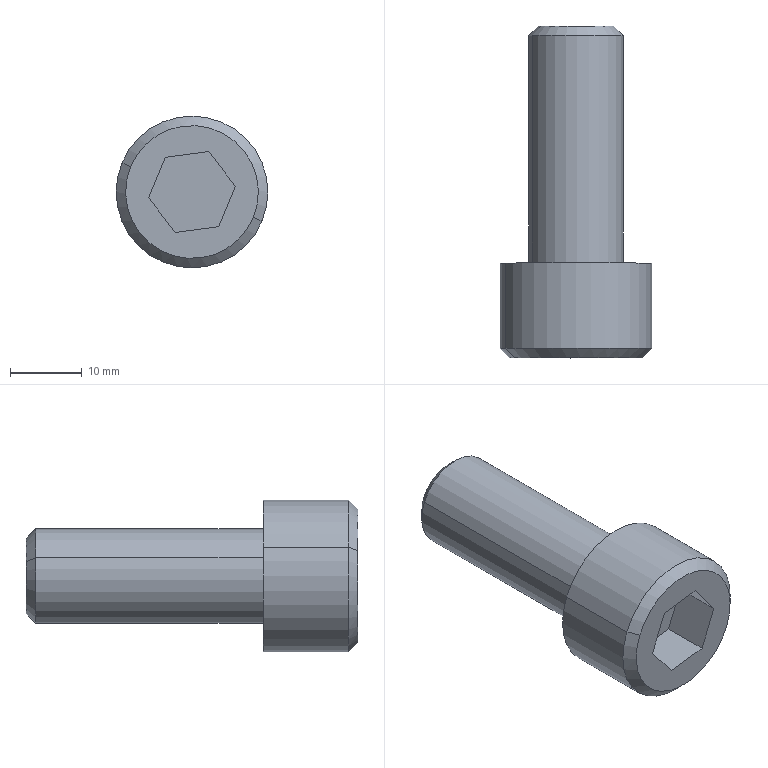Part | SolidWorks | features BaseBody 1 | 1 solid | 18 faces | box 21.12 x 46.2 x 21.12 mm | volume 8414 mm3 | plane 10 | cone 4 | cylinder 4 | commonest cylinder face diameters 13.2 x2 21.12 x2
STEP:
#1=CARTESIAN_POINT('',(-2171.446,543.257,-1544.855));
#2=VERTEX_POINT('',#1);
#3=CARTESIAN_POINT('',(-2170.226,541.937,-1545.359));
#4=VERTEX_POINT('',#3);
#5=CARTESIAN_POINT('',(-2171.446,543.257,-1544.855));
#6=DIRECTION('',(0.6535,-0.7071,-0.27));
#7=VECTOR('',#6,1000.);
#8=LINE('',#5,#7);
#9=EDGE_CURVE('',#2,#4,#8,.T.);
#10=ORIENTED_EDGE('',*,*,#9,.T.);
#11=CARTESIAN_POINT('',(-2153.147,541.937,-1552.416));
#12=VERTEX_POINT('',#11);
#13=CARTESIAN_POINT('',(-2161.687,541.937,-1548.888));
#14=DIRECTION('',(0.,-1.,0.));
#15=DIRECTION('',(0.9242,0.,-0.3818));
#16=AXIS2_PLACEMENT_3D('',#13,#14,#15);
#17=CIRCLE('',#16,9.24);
#18=EDGE_CURVE('',#12,#4,#17,.T.);
#19=ORIENTED_EDGE('',*,*,#18,.F.);
#20=CARTESIAN_POINT('',(-2151.927,543.257,-1552.92));
#21=VERTEX_POINT('',#20);
#22=CARTESIAN_POINT('',(-2153.147,541.937,-1552.416));
#23=DIRECTION('',(0.6535,0.7071,-0.27));
#24=VECTOR('',#23,1000.);
#25=LINE('',#22,#24);
#26=EDGE_CURVE('',#12,#21,#25,.T.);
#27=ORIENTED_EDGE('',*,*,#26,.T.);
#28=CARTESIAN_POINT('',(-2161.687,543.257,-1548.888));
#29=DIRECTION('',(0.,1.,0.));
#30=DIRECTION('',(-0.9242,0.,0.3818));
#31=AXIS2_PLACEMENT_3D('',#28,#29,#30);
#32=CIRCLE('',#31,10.56);
#33=EDGE_CURVE('',#2,#21,#32,.T.);
#34=ORIENTED_EDGE('',*,*,#33,.F.);
#35=EDGE_LOOP('',(#10,#19,#27,#34));
#36=FACE_OUTER_BOUND('',#35,.T.);
#37=CARTESIAN_POINT('',(-2161.687,541.871,-1548.888));
#38=DIRECTION('',(0.,1.,0.));
#39=DIRECTION('',(-0.954,0.,0.2998));
#40=AXIS2_PLACEMENT_3D('',#37,#38,#39);
#41=CONICAL_SURFACE('',#40,9.174,0.7854);
#42=ADVANCED_FACE('',(#36),#41,.T.);
#43=CARTESIAN_POINT('',(-2156.807,588.137,-1550.904));
#44=VERTEX_POINT('',#43);
#45=CARTESIAN_POINT('',(-2155.587,586.817,-1551.408));
#46=VERTEX_POINT('',#45);
#47=CARTESIAN_POINT('',(-2156.807,588.137,-1550.904));
#48=DIRECTION('',(0.6535,-0.7071,-0.27));
#49=VECTOR('',#48,1000.);
#50=LINE('',#47,#49);
#51=EDGE_CURVE('',#44,#46,#50,.T.);
#52=ORIENTED_EDGE('',*,*,#51,.T.);
#53=CARTESIAN_POINT('',(-2167.786,586.817,-1546.367));
#54=VERTEX_POINT('',#53);
#55=CARTESIAN_POINT('',(-2161.687,586.817,-1548.888));
#56=DIRECTION('',(0.,-1.,0.));
#57=DIRECTION('',(-0.9242,0.,0.3818));
#58=AXIS2_PLACEMENT_3D('',#55,#56,#57);
#59=CIRCLE('',#58,6.6);
#60=EDGE_CURVE('',#54,#46,#59,.T.);
#61=ORIENTED_EDGE('',*,*,#60,.F.);
#62=CARTESIAN_POINT('',(-2166.566,588.137,-1546.871));
#63=VERTEX_POINT('',#62);
#64=CARTESIAN_POINT('',(-2167.786,586.817,-1546.367));
#65=DIRECTION('',(0.6535,0.7071,-0.27));
#66=VECTOR('',#65,1000.);
#67=LINE('',#64,#66);
#68=EDGE_CURVE('',#54,#63,#67,.T.);
#69=ORIENTED_EDGE('',*,*,#68,.T.);
#70=CARTESIAN_POINT('',(-2161.687,588.137,-1548.888));
#71=DIRECTION('',(0.,1.,0.));
#72=DIRECTION('',(0.9242,0.,-0.3818));
#73=AXIS2_PLACEMENT_3D('',#70,#71,#72);
#74=CIRCLE('',#73,5.28);
#75=EDGE_CURVE('',#44,#63,#74,.T.);
#76=ORIENTED_EDGE('',*,*,#75,.F.);
#77=EDGE_LOOP('',(#52,#61,#69,#76));
#78=FACE_OUTER_BOUND('',#77,.T.);
#79=CARTESIAN_POINT('',(-2161.687,588.203,-1548.888));
#80=DIRECTION('',(0.,-1.,0.));
#81=DIRECTION('',(-0.8874,0.,0.4609));
#82=AXIS2_PLACEMENT_3D('',#79,#80,#81);
#83=CONICAL_SURFACE('',#82,5.214,0.7854);
#84=ADVANCED_FACE('',(#78),#83,.T.);
#85=CARTESIAN_POINT('',(-2167.786,555.137,-1546.367));
#86=VERTEX_POINT('',#85);
#87=CARTESIAN_POINT('',(-2167.786,555.137,-1546.367));
#88=DIRECTION('',(0.,1.,0.));
#89=VECTOR('',#88,1000.);
#90=LINE('',#87,#89);
#91=EDGE_CURVE('',#86,#54,#90,.T.);
#92=ORIENTED_EDGE('',*,*,#91,.T.);
#93=ORIENTED_EDGE('',*,*,#60,.T.);
#94=CARTESIAN_POINT('',(-2155.587,555.137,-1551.408));
#95=VERTEX_POINT('',#94);
#96=CARTESIAN_POINT('',(-2155.587,586.817,-1551.408));
#97=DIRECTION('',(0.,-1.,0.));
#98=VECTOR('',#97,1000.);
#99=LINE('',#96,#98);
#100=EDGE_CURVE('',#46,#95,#99,.T.);
#101=ORIENTED_EDGE('',*,*,#100,.T.);
#102=CARTESIAN_POINT('',(-2161.687,555.137,-1548.888));
#103=DIRECTION('',(0.,1.,0.));
#104=DIRECTION('',(0.9242,0.,-0.3818));
#105=AXIS2_PLACEMENT_3D('',#102,#103,#104);
#106=CIRCLE('',#105,6.6);
#107=EDGE_CURVE('',#95,#86,#106,.T.);
#108=ORIENTED_EDGE('',*,*,#107,.T.);
#109=EDGE_LOOP('',(#92,#93,#101,#108));
#110=FACE_OUTER_BOUND('',#109,.T.);
#111=CARTESIAN_POINT('',(-2161.687,588.401,-1548.888));
#112=DIRECTION('',(0.,1.,0.));
#113=DIRECTION('',(0.954,0.,-0.2998));
#114=AXIS2_PLACEMENT_3D('',#111,#112,#113);
#115=CYLINDRICAL_SURFACE('',#114,6.6);
#116=ADVANCED_FACE('',(#110),#115,.T.);
#117=CARTESIAN_POINT('',(-2151.927,555.137,-1552.92));
#118=VERTEX_POINT('',#117);
#119=CARTESIAN_POINT('',(-2151.927,555.137,-1552.92));
#120=DIRECTION('',(0.,-1.,0.));
#121=VECTOR('',#120,1000.);
#122=LINE('',#119,#121);
#123=EDGE_CURVE('',#118,#21,#122,.T.);
#124=ORIENTED_EDGE('',*,*,#123,.T.);
#125=CARTESIAN_POINT('',(-2161.687,543.257,-1548.888));
#126=DIRECTION('',(0.,1.,0.));
#127=DIRECTION('',(0.9242,0.,-0.3818));
#128=AXIS2_PLACEMENT_3D('',#125,#126,#127);
#129=CIRCLE('',#128,10.56);
#130=EDGE_CURVE('',#21,#2,#129,.T.);
#131=ORIENTED_EDGE('',*,*,#130,.T.);
#132=CARTESIAN_POINT('',(-2171.446,555.137,-1544.855));
#133=VERTEX_POINT('',#132);
#134=CARTESIAN_POINT('',(-2171.446,543.257,-1544.855));
#135=DIRECTION('',(0.,1.,0.));
#136=VECTOR('',#135,1000.);
#137=LINE('',#134,#136);
#138=EDGE_CURVE('',#2,#133,#137,.T.);
#139=ORIENTED_EDGE('',*,*,#138,.T.);
#140=CARTESIAN_POINT('',(-2161.687,555.137,-1548.888));
#141=DIRECTION('',(0.,1.,0.));
#142=DIRECTION('',(0.9242,0.,-0.3818));
#143=AXIS2_PLACEMENT_3D('',#140,#141,#142);
#144=CIRCLE('',#143,10.56);
#145=EDGE_CURVE('',#118,#133,#144,.T.);
#146=ORIENTED_EDGE('',*,*,#145,.F.);
#147=EDGE_LOOP('',(#124,#131,#139,#146));
#148=FACE_OUTER_BOUND('',#147,.T.);
#149=CARTESIAN_POINT('',(-2161.687,542.663,-1548.888));
#150=DIRECTION('',(0.,-1.,0.));
#151=DIRECTION('',(-0.8874,0.,0.4609));
#152=AXIS2_PLACEMENT_3D('',#149,#150,#151);
#153=CYLINDRICAL_SURFACE('',#152,10.56);
#154=ADVANCED_FACE('',(#148),#153,.T.);
#155=CARTESIAN_POINT('',(-2155.643,548.537,-1548.086));
#156=VERTEX_POINT('',#155);
#157=CARTESIAN_POINT('',(-2159.358,548.537,-1543.253));
#158=VERTEX_POINT('',#157);
#159=CARTESIAN_POINT('',(-2155.643,548.537,-1548.086));
#160=DIRECTION('',(-0.6095,0.,0.7928));
#161=VECTOR('',#160,1000.);
#162=LINE('',#159,#161);
#163=EDGE_CURVE('',#156,#158,#162,.T.);
#164=ORIENTED_EDGE('',*,*,#163,.T.);
#165=CARTESIAN_POINT('',(-2165.402,548.537,-1544.054));
#166=VERTEX_POINT('',#165);
#167=CARTESIAN_POINT('',(-2159.358,548.537,-1543.253));
#168=DIRECTION('',(-0.9913,0.,-0.1314));
#169=VECTOR('',#168,1000.);
#170=LINE('',#167,#169);
#171=EDGE_CURVE('',#158,#166,#170,.T.);
#172=ORIENTED_EDGE('',*,*,#171,.T.);
#173=CARTESIAN_POINT('',(-2167.73,548.537,-1549.689));
#174=VERTEX_POINT('',#173);
#175=CARTESIAN_POINT('',(-2165.402,548.537,-1544.054));
#176=DIRECTION('',(-0.3818,0.,-0.9242));
#177=VECTOR('',#176,1000.);
#178=LINE('',#175,#177);
#179=EDGE_CURVE('',#166,#174,#178,.T.);
#180=ORIENTED_EDGE('',*,*,#179,.T.);
#181=CARTESIAN_POINT('',(-2164.015,548.537,-1554.522));
#182=VERTEX_POINT('',#181);
#183=CARTESIAN_POINT('',(-2167.73,548.537,-1549.689));
#184=DIRECTION('',(0.6095,0.,-0.7928));
#185=VECTOR('',#184,1000.);
#186=LINE('',#183,#185);
#187=EDGE_CURVE('',#174,#182,#186,.T.);
#188=ORIENTED_EDGE('',*,*,#187,.T.);
#189=CARTESIAN_POINT('',(-2157.971,548.537,-1553.721));
#190=VERTEX_POINT('',#189);
#191=CARTESIAN_POINT('',(-2164.015,548.537,-1554.522));
#192=DIRECTION('',(0.9913,0.,0.1314));
#193=VECTOR('',#192,1000.);
#194=LINE('',#191,#193);
#195=EDGE_CURVE('',#182,#190,#194,.T.);
#196=ORIENTED_EDGE('',*,*,#195,.T.);
#197=CARTESIAN_POINT('',(-2157.971,548.537,-1553.721));
#198=DIRECTION('',(0.3818,0.,0.9242));
#199=VECTOR('',#198,1000.);
#200=LINE('',#197,#199);
#201=EDGE_CURVE('',#190,#156,#200,.T.);
#202=ORIENTED_EDGE('',*,*,#201,.T.);
#203=EDGE_LOOP('',(#164,#172,#180,#188,#196,#202));
#204=FACE_OUTER_BOUND('',#203,.T.);
#205=CARTESIAN_POINT('',(-2153.682,548.537,-1544.938));
#206=DIRECTION('',(0.,-1.,0.));
#207=DIRECTION('',(0.,0.,-1.));
#208=AXIS2_PLACEMENT_3D('',#205,#206,#207);
#209=PLANE('',#208);
#210=ADVANCED_FACE('',(#204),#209,.T.);
#211=CARTESIAN_POINT('',(-2157.971,541.937,-1553.721));
#212=VERTEX_POINT('',#211);
#213=CARTESIAN_POINT('',(-2155.643,541.937,-1548.086));
#214=VERTEX_POINT('',#213);
#215=CARTESIAN_POINT('',(-2157.971,541.937,-1553.721));
#216=DIRECTION('',(0.3818,0.,0.9242));
#217=VECTOR('',#216,1000.);
#218=LINE('',#215,#217);
#219=EDGE_CURVE('',#212,#214,#218,.T.);
#220=ORIENTED_EDGE('',*,*,#219,.T.);
#221=CARTESIAN_POINT('',(-2155.643,548.537,-1548.086));
#222=DIRECTION('',(0.,-1.,0.));
#223=VECTOR('',#222,1000.);
#224=LINE('',#221,#223);
#225=EDGE_CURVE('',#156,#214,#224,.T.);
#226=ORIENTED_EDGE('',*,*,#225,.F.);
#227=ORIENTED_EDGE('',*,*,#201,.F.);
#228=CARTESIAN_POINT('',(-2157.971,548.537,-1553.721));
#229=DIRECTION('',(0.,-1.,0.));
#230=VECTOR('',#229,1000.);
#231=LINE('',#228,#230);
#232=EDGE_CURVE('',#190,#212,#231,.T.);
#233=ORIENTED_EDGE('',*,*,#232,.T.);
#234=EDGE_LOOP('',(#220,#226,#227,#233));
#235=FACE_OUTER_BOUND('',#234,.T.);
#236=CARTESIAN_POINT('',(-2158.097,541.607,-1554.026));
#237=DIRECTION('',(-0.9242,0.,0.3818));
#238=DIRECTION('',(0.,1.,0.));
#239=AXIS2_PLACEMENT_3D('',#236,#237,#238);
#240=PLANE('',#239);
#241=ADVANCED_FACE('',(#235),#240,.T.);
#242=CARTESIAN_POINT('',(-2164.015,541.937,-1554.522));
#243=VERTEX_POINT('',#242);
#244=CARTESIAN_POINT('',(-2164.015,541.937,-1554.522));
#245=DIRECTION('',(0.9913,0.,0.1314));
#246=VECTOR('',#245,1000.);
#247=LINE('',#244,#246);
#248=EDGE_CURVE('',#243,#212,#247,.T.);
#249=ORIENTED_EDGE('',*,*,#248,.T.);
#250=ORIENTED_EDGE('',*,*,#232,.F.);
#251=ORIENTED_EDGE('',*,*,#195,.F.);
#252=CARTESIAN_POINT('',(-2164.015,548.537,-1554.522));
#253=DIRECTION('',(0.,-1.,0.));
#254=VECTOR('',#253,1000.);
#255=LINE('',#252,#254);
#256=EDGE_CURVE('',#182,#243,#255,.T.);
#257=ORIENTED_EDGE('',*,*,#256,.T.);
#258=EDGE_LOOP('',(#249,#250,#251,#257));
#259=FACE_OUTER_BOUND('',#258,.T.);
#260=CARTESIAN_POINT('',(-2164.342,541.607,-1554.566));
#261=DIRECTION('',(-0.1314,0.,0.9913));
#262=DIRECTION('',(0.,1.,0.));
#263=AXIS2_PLACEMENT_3D('',#260,#261,#262);
#264=PLANE('',#263);
#265=ADVANCED_FACE('',(#259),#264,.T.);
#266=CARTESIAN_POINT('',(-2167.73,541.937,-1549.689));
#267=VERTEX_POINT('',#266);
#268=CARTESIAN_POINT('',(-2167.73,541.937,-1549.689));
#269=DIRECTION('',(0.6095,0.,-0.7928));
#270=VECTOR('',#269,1000.);
#271=LINE('',#268,#270);
#272=EDGE_CURVE('',#267,#243,#271,.T.);
#273=ORIENTED_EDGE('',*,*,#272,.T.);
#274=ORIENTED_EDGE('',*,*,#256,.F.);
#275=ORIENTED_EDGE('',*,*,#187,.F.);
#276=CARTESIAN_POINT('',(-2167.73,548.537,-1549.689));
#277=DIRECTION('',(0.,-1.,0.));
#278=VECTOR('',#277,1000.);
#279=LINE('',#276,#278);
#280=EDGE_CURVE('',#174,#267,#279,.T.);
#281=ORIENTED_EDGE('',*,*,#280,.T.);
#282=EDGE_LOOP('',(#273,#274,#275,#281));
#283=FACE_OUTER_BOUND('',#282,.T.);
#284=CARTESIAN_POINT('',(-2167.932,541.607,-1549.427));
#285=DIRECTION('',(0.7928,0.,0.6095));
#286=DIRECTION('',(0.,-1.,0.));
#287=AXIS2_PLACEMENT_3D('',#284,#285,#286);
#288=PLANE('',#287);
#289=ADVANCED_FACE('',(#283),#288,.T.);
#290=CARTESIAN_POINT('',(-2165.402,541.937,-1544.054));
#291=VERTEX_POINT('',#290);
#292=CARTESIAN_POINT('',(-2165.402,541.937,-1544.054));
#293=DIRECTION('',(-0.3818,0.,-0.9242));
#294=VECTOR('',#293,1000.);
#295=LINE('',#292,#294);
#296=EDGE_CURVE('',#291,#267,#295,.T.);
#297=ORIENTED_EDGE('',*,*,#296,.T.);
#298=ORIENTED_EDGE('',*,*,#280,.F.);
#299=ORIENTED_EDGE('',*,*,#179,.F.);
#300=CARTESIAN_POINT('',(-2165.402,548.537,-1544.054));
#301=DIRECTION('',(0.,-1.,0.));
#302=VECTOR('',#301,1000.);
#303=LINE('',#300,#302);
#304=EDGE_CURVE('',#166,#291,#303,.T.);
#305=ORIENTED_EDGE('',*,*,#304,.T.);
#306=EDGE_LOOP('',(#297,#298,#299,#305));
#307=FACE_OUTER_BOUND('',#306,.T.);
#308=CARTESIAN_POINT('',(-2165.276,541.607,-1543.749));
#309=DIRECTION('',(0.9242,0.,-0.3818));
#310=DIRECTION('',(0.,-1.,0.));
#311=AXIS2_PLACEMENT_3D('',#308,#309,#310);
#312=PLANE('',#311);
#313=ADVANCED_FACE('',(#307),#312,.T.);
#314=CARTESIAN_POINT('',(-2159.358,541.937,-1543.253));
#315=VERTEX_POINT('',#314);
#316=CARTESIAN_POINT('',(-2159.358,541.937,-1543.253));
#317=DIRECTION('',(-0.9913,0.,-0.1314));
#318=VECTOR('',#317,1000.);
#319=LINE('',#316,#318);
#320=EDGE_CURVE('',#315,#291,#319,.T.);
#321=ORIENTED_EDGE('',*,*,#320,.T.);
#322=ORIENTED_EDGE('',*,*,#304,.F.);
#323=ORIENTED_EDGE('',*,*,#171,.F.);
#324=CARTESIAN_POINT('',(-2159.358,548.537,-1543.253));
#325=DIRECTION('',(0.,-1.,0.));
#326=VECTOR('',#325,1000.);
#327=LINE('',#324,#326);
#328=EDGE_CURVE('',#158,#315,#327,.T.);
#329=ORIENTED_EDGE('',*,*,#328,.T.);
#330=EDGE_LOOP('',(#321,#322,#323,#329));
#331=FACE_OUTER_BOUND('',#330,.T.);
#332=CARTESIAN_POINT('',(-2159.031,541.607,-1543.209));
#333=DIRECTION('',(0.1314,0.,-0.9913));
#334=DIRECTION('',(0.,-1.,0.));
#335=AXIS2_PLACEMENT_3D('',#332,#333,#334);
#336=PLANE('',#335);
#337=ADVANCED_FACE('',(#331),#336,.T.);
#338=CARTESIAN_POINT('',(-2155.643,541.937,-1548.086));
#339=DIRECTION('',(-0.6095,0.,0.7928));
#340=VECTOR('',#339,1000.);
#341=LINE('',#338,#340);
#342=EDGE_CURVE('',#214,#315,#341,.T.);
#343=ORIENTED_EDGE('',*,*,#342,.T.);
#344=ORIENTED_EDGE('',*,*,#328,.F.);
#345=ORIENTED_EDGE('',*,*,#163,.F.);
#346=ORIENTED_EDGE('',*,*,#225,.T.);
#347=EDGE_LOOP('',(#343,#344,#345,#346));
#348=FACE_OUTER_BOUND('',#347,.T.);
#349=CARTESIAN_POINT('',(-2155.441,541.607,-1548.348));
#350=DIRECTION('',(-0.7928,0.,-0.6095));
#351=DIRECTION('',(-0.6095,0.,0.7928));
#352=AXIS2_PLACEMENT_3D('',#349,#350,#351);
#353=PLANE('',#352);
#354=ADVANCED_FACE('',(#348),#353,.T.);
#355=ORIENTED_EDGE('',*,*,#26,.F.);
#356=CARTESIAN_POINT('',(-2161.687,541.937,-1548.888));
#357=DIRECTION('',(0.,-1.,0.));
#358=DIRECTION('',(-0.9242,0.,0.3818));
#359=AXIS2_PLACEMENT_3D('',#356,#357,#358);
#360=CIRCLE('',#359,9.24);
#361=EDGE_CURVE('',#4,#12,#360,.T.);
#362=ORIENTED_EDGE('',*,*,#361,.F.);
#363=ORIENTED_EDGE('',*,*,#9,.F.);
#364=ORIENTED_EDGE('',*,*,#130,.F.);
#365=EDGE_LOOP('',(#355,#362,#363,#364));
#366=FACE_OUTER_BOUND('',#365,.T.);
#367=CARTESIAN_POINT('',(-2161.687,541.871,-1548.888));
#368=DIRECTION('',(0.,1.,0.));
#369=DIRECTION('',(0.954,0.,-0.2998));
#370=AXIS2_PLACEMENT_3D('',#367,#368,#369);
#371=CONICAL_SURFACE('',#370,9.174,0.7854);
#372=ADVANCED_FACE('',(#366),#371,.T.);
#373=ORIENTED_EDGE('',*,*,#68,.F.);
#374=CARTESIAN_POINT('',(-2161.687,586.817,-1548.888));
#375=DIRECTION('',(0.,-1.,0.));
#376=DIRECTION('',(0.9242,0.,-0.3818));
#377=AXIS2_PLACEMENT_3D('',#374,#375,#376);
#378=CIRCLE('',#377,6.6);
#379=EDGE_CURVE('',#46,#54,#378,.T.);
#380=ORIENTED_EDGE('',*,*,#379,.F.);
#381=ORIENTED_EDGE('',*,*,#51,.F.);
#382=CARTESIAN_POINT('',(-2161.687,588.137,-1548.888));
#383=DIRECTION('',(0.,1.,0.));
#384=DIRECTION('',(-0.9242,0.,0.3818));
#385=AXIS2_PLACEMENT_3D('',#382,#383,#384);
#386=CIRCLE('',#385,5.28);
#387=EDGE_CURVE('',#63,#44,#386,.T.);
#388=ORIENTED_EDGE('',*,*,#387,.F.);
#389=EDGE_LOOP('',(#373,#380,#381,#388));
#390=FACE_OUTER_BOUND('',#389,.T.);
#391=CARTESIAN_POINT('',(-2161.687,588.203,-1548.888));
#392=DIRECTION('',(0.,-1.,0.));
#393=DIRECTION('',(0.8874,0.,-0.4609));
#394=AXIS2_PLACEMENT_3D('',#391,#392,#393);
#395=CONICAL_SURFACE('',#394,5.214,0.7854);
#396=ADVANCED_FACE('',(#390),#395,.T.);
#397=ORIENTED_EDGE('',*,*,#100,.F.);
#398=ORIENTED_EDGE('',*,*,#379,.T.);
#399=ORIENTED_EDGE('',*,*,#91,.F.);
#400=CARTESIAN_POINT('',(-2161.687,555.137,-1548.888));
#401=DIRECTION('',(0.,1.,0.));
#402=DIRECTION('',(-0.9242,0.,0.3818));
#403=AXIS2_PLACEMENT_3D('',#400,#401,#402);
#404=CIRCLE('',#403,6.6);
#405=EDGE_CURVE('',#86,#95,#404,.T.);
#406=ORIENTED_EDGE('',*,*,#405,.T.);
#407=EDGE_LOOP('',(#397,#398,#399,#406));
#408=FACE_OUTER_BOUND('',#407,.T.);
#409=CARTESIAN_POINT('',(-2161.687,588.401,-1548.888));
#410=DIRECTION('',(0.,1.,0.));
#411=DIRECTION('',(-0.954,0.,0.2998));
#412=AXIS2_PLACEMENT_3D('',#409,#410,#411);
#413=CYLINDRICAL_SURFACE('',#412,6.6);
#414=ADVANCED_FACE('',(#408),#413,.T.);
#415=ORIENTED_EDGE('',*,*,#75,.T.);
#416=ORIENTED_EDGE('',*,*,#387,.T.);
#417=EDGE_LOOP('',(#415,#416));
#418=FACE_OUTER_BOUND('',#417,.T.);
#419=CARTESIAN_POINT('',(-2158.516,588.137,-1556.424));
#420=DIRECTION('',(0.,1.,0.));
#421=DIRECTION('',(1.,0.,0.));
#422=AXIS2_PLACEMENT_3D('',#419,#420,#421);
#423=PLANE('',#422);
#424=ADVANCED_FACE('',(#418),#423,.T.);
#425=ORIENTED_EDGE('',*,*,#138,.F.);
#426=ORIENTED_EDGE('',*,*,#33,.T.);
#427=ORIENTED_EDGE('',*,*,#123,.F.);
#428=CARTESIAN_POINT('',(-2161.687,555.137,-1548.888));
#429=DIRECTION('',(0.,1.,0.));
#430=DIRECTION('',(-0.9242,0.,0.3818));
#431=AXIS2_PLACEMENT_3D('',#428,#429,#430);
#432=CIRCLE('',#431,10.56);
#433=EDGE_CURVE('',#133,#118,#432,.T.);
#434=ORIENTED_EDGE('',*,*,#433,.F.);
#435=EDGE_LOOP('',(#425,#426,#427,#434));
#436=FACE_OUTER_BOUND('',#435,.T.);
#437=CARTESIAN_POINT('',(-2161.687,542.663,-1548.888));
#438=DIRECTION('',(0.,-1.,0.));
#439=DIRECTION('',(0.8874,0.,-0.4609));
#440=AXIS2_PLACEMENT_3D('',#437,#438,#439);
#441=CYLINDRICAL_SURFACE('',#440,10.56);
#442=ADVANCED_FACE('',(#436),#441,.T.);
#443=ORIENTED_EDGE('',*,*,#107,.F.);
#444=ORIENTED_EDGE('',*,*,#405,.F.);
#445=EDGE_LOOP('',(#443,#444));
#446=FACE_BOUND('',#445,.T.);
#447=ORIENTED_EDGE('',*,*,#145,.T.);
#448=ORIENTED_EDGE('',*,*,#433,.T.);
#449=EDGE_LOOP('',(#447,#448));
#450=FACE_OUTER_BOUND('',#449,.T.);
#451=CARTESIAN_POINT('',(-2155.382,555.137,-1564.045));
#452=DIRECTION('',(0.,1.,0.));
#453=DIRECTION('',(1.,0.,0.));
#454=AXIS2_PLACEMENT_3D('',#451,#452,#453);
#455=PLANE('',#454);
#456=ADVANCED_FACE('',(#446,#450),#455,.T.);
#457=ORIENTED_EDGE('',*,*,#342,.F.);
#458=ORIENTED_EDGE('',*,*,#219,.F.);
#459=ORIENTED_EDGE('',*,*,#248,.F.);
#460=ORIENTED_EDGE('',*,*,#272,.F.);
#461=ORIENTED_EDGE('',*,*,#296,.F.);
#462=ORIENTED_EDGE('',*,*,#320,.F.);
#463=EDGE_LOOP('',(#457,#458,#459,#460,#461,#462));
#464=FACE_BOUND('',#463,.T.);
#465=ORIENTED_EDGE('',*,*,#361,.T.);
#466=ORIENTED_EDGE('',*,*,#18,.T.);
#467=EDGE_LOOP('',(#465,#466));
#468=FACE_OUTER_BOUND('',#467,.T.);
#469=CARTESIAN_POINT('',(-2174.904,541.937,-1554.408));
#470=DIRECTION('',(0.,-1.,0.));
#471=DIRECTION('',(0.,0.,-1.));
#472=AXIS2_PLACEMENT_3D('',#469,#470,#471);
#473=PLANE('',#472);
#474=ADVANCED_FACE('',(#464,#468),#473,.T.);
#475=CLOSED_SHELL('',(#42,#84,#116,#154,#210,#241,#265,#289,#313,#337,#354,#372,#396,#414,#424,#442,#456,#474));
#476=MANIFOLD_SOLID_BREP('',#475);
#477=CARTESIAN_POINT('',(0.,0.,0.));
#478=DIRECTION('',(0.,0.,1.));
#479=DIRECTION('',(1.,0.,0.));
#480=AXIS2_PLACEMENT_3D('',#477,#478,#479);
#481=(LENGTH_UNIT()NAMED_UNIT(*)SI_UNIT(.MILLI.,.METRE.));
#482=UNCERTAINTY_MEASURE_WITH_UNIT(LENGTH_MEASURE(0.00001),#481,'','');
#483=(NAMED_UNIT(*)PLANE_ANGLE_UNIT()SI_UNIT($,.RADIAN.));
#484=(NAMED_UNIT(*)SI_UNIT($,.STERADIAN.)SOLID_ANGLE_UNIT());
#485=(GEOMETRIC_REPRESENTATION_CONTEXT(3)GLOBAL_UNCERTAINTY_ASSIGNED_CONTEXT((#482))GLOBAL_UNIT_ASSIGNED_CONTEXT((#481,#483,#484))REPRESENTATION_CONTEXT('',''));
#486=ADVANCED_BREP_SHAPE_REPRESENTATION('',(#476,#480),#485);